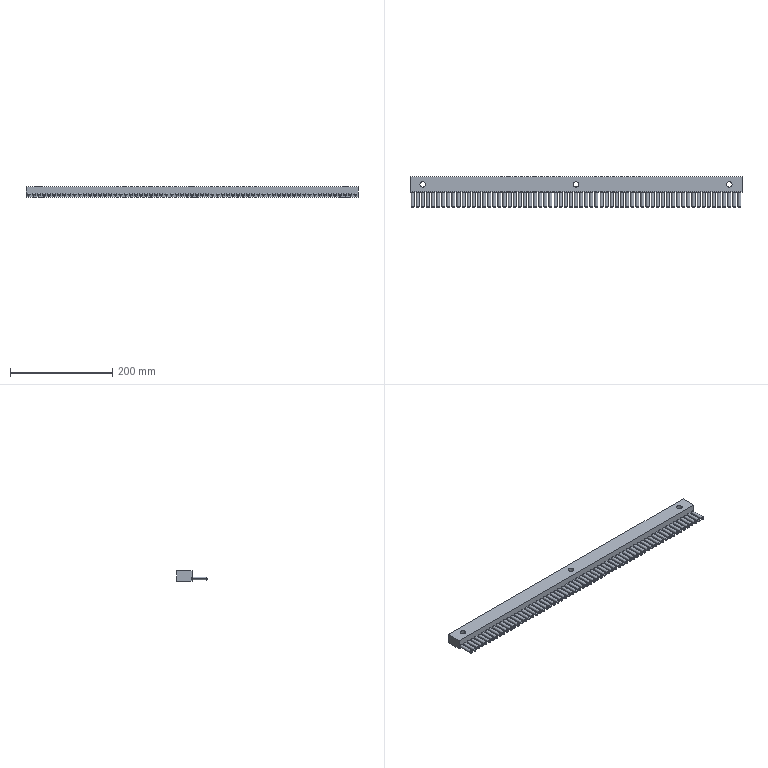Part | SolidWorks | features ICE 3, Fillet 2, Extrusion 1, LPattern 1, Sweep 1 | 1 solid | 346 faces | box 650 x 60 x 20 mm | volume 429985 mm3 | cylinder 142 | torus 130 | plane 74 | commonest cylinder face diameters 6 x130 11 x6 22 x6